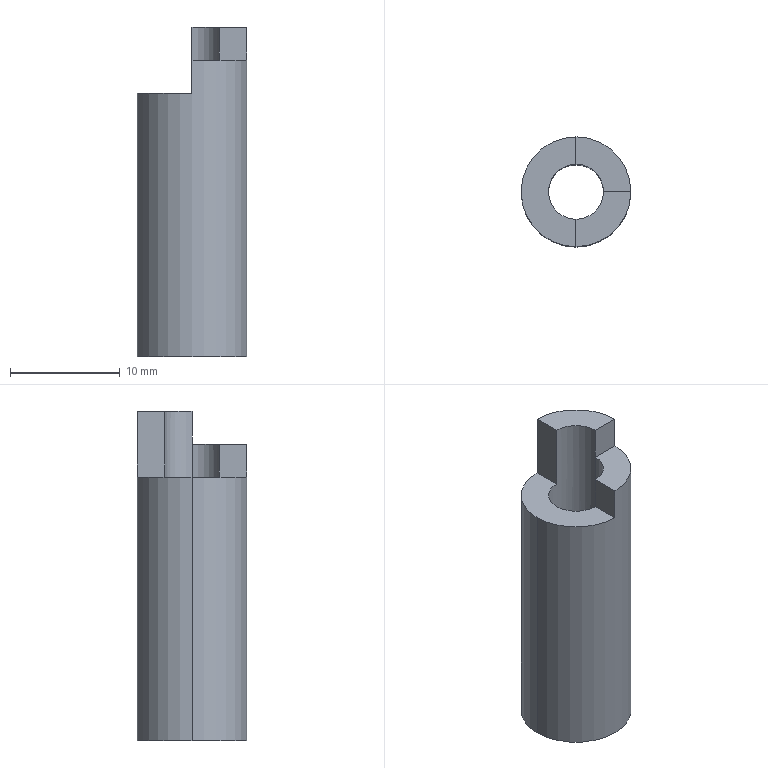Part | SolidWorks | features BaseBody 1 | 1 solid | 11 faces | box 10 x 10 x 30 mm | volume 1546 mm3 | plane 7 | cylinder 4 | commonest cylinder face diameters 5.003 x2 10 x2
STEP:
#1=CARTESIAN_POINT('',(-86.,-22.498,-9.829));
#2=VERTEX_POINT('',#1);
#3=CARTESIAN_POINT('',(-88.501,-25.,-9.829));
#4=VERTEX_POINT('',#3);
#5=CARTESIAN_POINT('',(-86.,-25.,-9.829));
#6=DIRECTION('',(0.,0.,1.));
#7=DIRECTION('',(-1.,0.,0.));
#8=AXIS2_PLACEMENT_3D('',#5,#6,#7);
#9=CIRCLE('',#8,2.502);
#10=EDGE_CURVE('',#2,#4,#9,.T.);
#11=ORIENTED_EDGE('',*,*,#10,.T.);
#12=CARTESIAN_POINT('',(-88.501,-25.,-33.829));
#13=VERTEX_POINT('',#12);
#14=CARTESIAN_POINT('',(-88.501,-25.,-3.829));
#15=DIRECTION('',(0.,0.,-1.));
#16=VECTOR('',#15,1000.);
#17=LINE('',#14,#16);
#18=EDGE_CURVE('',#4,#13,#17,.T.);
#19=ORIENTED_EDGE('',*,*,#18,.T.);
#20=CARTESIAN_POINT('',(-83.498,-25.,-33.829));
#21=VERTEX_POINT('',#20);
#22=CARTESIAN_POINT('',(-86.,-25.,-33.829));
#23=DIRECTION('',(0.,0.,1.));
#24=DIRECTION('',(1.,0.,0.));
#25=AXIS2_PLACEMENT_3D('',#22,#23,#24);
#26=CIRCLE('',#25,2.502);
#27=EDGE_CURVE('',#21,#13,#26,.T.);
#28=ORIENTED_EDGE('',*,*,#27,.F.);
#29=CARTESIAN_POINT('',(-83.499,-25.,-6.829));
#30=VERTEX_POINT('',#29);
#31=CARTESIAN_POINT('',(-83.498,-25.,-3.829));
#32=DIRECTION('',(0.,0.,-1.));
#33=VECTOR('',#32,1000.);
#34=LINE('',#31,#33);
#35=EDGE_CURVE('',#30,#21,#34,.T.);
#36=ORIENTED_EDGE('',*,*,#35,.F.);
#37=CARTESIAN_POINT('',(-83.499,-25.,-3.829));
#38=VERTEX_POINT('',#37);
#39=CARTESIAN_POINT('',(-83.499,-25.,-3.829));
#40=DIRECTION('',(0.,0.,1.));
#41=VECTOR('',#40,1000.);
#42=LINE('',#39,#41);
#43=EDGE_CURVE('',#30,#38,#42,.T.);
#44=ORIENTED_EDGE('',*,*,#43,.T.);
#45=CARTESIAN_POINT('',(-86.,-22.498,-3.829));
#46=VERTEX_POINT('',#45);
#47=CARTESIAN_POINT('',(-86.,-25.,-3.829));
#48=DIRECTION('',(0.,0.,-1.));
#49=DIRECTION('',(1.,0.,0.));
#50=AXIS2_PLACEMENT_3D('',#47,#48,#49);
#51=CIRCLE('',#50,2.502);
#52=EDGE_CURVE('',#46,#38,#51,.T.);
#53=ORIENTED_EDGE('',*,*,#52,.F.);
#54=CARTESIAN_POINT('',(-86.,-22.498,-3.829));
#55=DIRECTION('',(0.,0.,-1.));
#56=VECTOR('',#55,1000.);
#57=LINE('',#54,#56);
#58=EDGE_CURVE('',#46,#2,#57,.T.);
#59=ORIENTED_EDGE('',*,*,#58,.T.);
#60=EDGE_LOOP('',(#11,#19,#28,#36,#44,#53,#59));
#61=FACE_OUTER_BOUND('',#60,.T.);
#62=CARTESIAN_POINT('',(-86.,-25.,-3.829));
#63=DIRECTION('',(0.,0.,-1.));
#64=DIRECTION('',(1.,0.,0.));
#65=AXIS2_PLACEMENT_3D('',#62,#63,#64);
#66=CYLINDRICAL_SURFACE('',#65,2.502);
#67=ADVANCED_FACE('',(#61),#66,.F.);
#68=CARTESIAN_POINT('',(-91.,-25.,-9.829));
#69=VERTEX_POINT('',#68);
#70=CARTESIAN_POINT('',(-86.,-30.,-9.829));
#71=VERTEX_POINT('',#70);
#72=CARTESIAN_POINT('',(-86.,-25.,-9.829));
#73=DIRECTION('',(0.,0.,1.));
#74=DIRECTION('',(-1.,0.,0.));
#75=AXIS2_PLACEMENT_3D('',#72,#73,#74);
#76=CIRCLE('',#75,5.);
#77=EDGE_CURVE('',#69,#71,#76,.T.);
#78=ORIENTED_EDGE('',*,*,#77,.F.);
#79=CARTESIAN_POINT('',(-91.,-25.,-33.829));
#80=VERTEX_POINT('',#79);
#81=CARTESIAN_POINT('',(-91.,-25.,-3.829));
#82=DIRECTION('',(0.,0.,-1.));
#83=VECTOR('',#82,1000.);
#84=LINE('',#81,#83);
#85=EDGE_CURVE('',#69,#80,#84,.T.);
#86=ORIENTED_EDGE('',*,*,#85,.T.);
#87=CARTESIAN_POINT('',(-81.,-25.,-33.829));
#88=VERTEX_POINT('',#87);
#89=CARTESIAN_POINT('',(-86.,-25.,-33.829));
#90=DIRECTION('',(0.,0.,1.));
#91=DIRECTION('',(1.,0.,0.));
#92=AXIS2_PLACEMENT_3D('',#89,#90,#91);
#93=CIRCLE('',#92,5.);
#94=EDGE_CURVE('',#80,#88,#93,.T.);
#95=ORIENTED_EDGE('',*,*,#94,.T.);
#96=CARTESIAN_POINT('',(-81.,-25.,-6.829));
#97=VERTEX_POINT('',#96);
#98=CARTESIAN_POINT('',(-81.,-25.,-3.829));
#99=DIRECTION('',(0.,0.,-1.));
#100=VECTOR('',#99,1000.);
#101=LINE('',#98,#100);
#102=EDGE_CURVE('',#97,#88,#101,.T.);
#103=ORIENTED_EDGE('',*,*,#102,.F.);
#104=CARTESIAN_POINT('',(-86.,-30.,-6.829));
#105=VERTEX_POINT('',#104);
#106=CARTESIAN_POINT('',(-86.,-25.,-6.829));
#107=DIRECTION('',(0.,0.,1.));
#108=DIRECTION('',(-1.,0.,0.));
#109=AXIS2_PLACEMENT_3D('',#106,#107,#108);
#110=CIRCLE('',#109,5.);
#111=EDGE_CURVE('',#105,#97,#110,.T.);
#112=ORIENTED_EDGE('',*,*,#111,.F.);
#113=CARTESIAN_POINT('',(-86.,-30.,-3.829));
#114=DIRECTION('',(0.,0.,1.));
#115=VECTOR('',#114,1000.);
#116=LINE('',#113,#115);
#117=EDGE_CURVE('',#71,#105,#116,.T.);
#118=ORIENTED_EDGE('',*,*,#117,.F.);
#119=EDGE_LOOP('',(#78,#86,#95,#103,#112,#118));
#120=FACE_OUTER_BOUND('',#119,.T.);
#121=CARTESIAN_POINT('',(-86.,-25.,-3.829));
#122=DIRECTION('',(0.,0.,-1.));
#123=DIRECTION('',(1.,0.,0.));
#124=AXIS2_PLACEMENT_3D('',#121,#122,#123);
#125=CYLINDRICAL_SURFACE('',#124,5.);
#126=ADVANCED_FACE('',(#120),#125,.T.);
#127=ORIENTED_EDGE('',*,*,#27,.T.);
#128=CARTESIAN_POINT('',(-86.,-25.,-33.829));
#129=DIRECTION('',(0.,0.,1.));
#130=DIRECTION('',(1.,0.,0.));
#131=AXIS2_PLACEMENT_3D('',#128,#129,#130);
#132=CIRCLE('',#131,2.502);
#133=EDGE_CURVE('',#13,#21,#132,.T.);
#134=ORIENTED_EDGE('',*,*,#133,.T.);
#135=EDGE_LOOP('',(#127,#134));
#136=FACE_BOUND('',#135,.T.);
#137=CARTESIAN_POINT('',(-86.,-25.,-33.829));
#138=DIRECTION('',(0.,0.,1.));
#139=DIRECTION('',(1.,0.,0.));
#140=AXIS2_PLACEMENT_3D('',#137,#138,#139);
#141=CIRCLE('',#140,5.);
#142=EDGE_CURVE('',#88,#80,#141,.T.);
#143=ORIENTED_EDGE('',*,*,#142,.F.);
#144=ORIENTED_EDGE('',*,*,#94,.F.);
#145=EDGE_LOOP('',(#143,#144));
#146=FACE_OUTER_BOUND('',#145,.T.);
#147=CARTESIAN_POINT('',(-86.,-25.,-33.829));
#148=DIRECTION('',(0.,0.,-1.));
#149=DIRECTION('',(-1.,0.,0.));
#150=AXIS2_PLACEMENT_3D('',#147,#148,#149);
#151=PLANE('',#150);
#152=ADVANCED_FACE('',(#136,#146),#151,.T.);
#153=CARTESIAN_POINT('',(-81.,-25.,-3.829));
#154=VERTEX_POINT('',#153);
#155=CARTESIAN_POINT('',(-86.,-25.,-3.829));
#156=DIRECTION('',(1.,0.,0.));
#157=VECTOR('',#156,1000.);
#158=LINE('',#155,#157);
#159=EDGE_CURVE('',#38,#154,#158,.T.);
#160=ORIENTED_EDGE('',*,*,#159,.T.);
#161=CARTESIAN_POINT('',(-86.,-20.,-3.829));
#162=VERTEX_POINT('',#161);
#163=CARTESIAN_POINT('',(-86.,-25.,-3.829));
#164=DIRECTION('',(0.,0.,-1.));
#165=DIRECTION('',(1.,0.,0.));
#166=AXIS2_PLACEMENT_3D('',#163,#164,#165);
#167=CIRCLE('',#166,5.);
#168=EDGE_CURVE('',#162,#154,#167,.T.);
#169=ORIENTED_EDGE('',*,*,#168,.F.);
#170=CARTESIAN_POINT('',(-86.,-25.,-3.829));
#171=DIRECTION('',(0.,-1.,0.));
#172=VECTOR('',#171,1000.);
#173=LINE('',#170,#172);
#174=EDGE_CURVE('',#162,#46,#173,.T.);
#175=ORIENTED_EDGE('',*,*,#174,.T.);
#176=ORIENTED_EDGE('',*,*,#52,.T.);
#177=EDGE_LOOP('',(#160,#169,#175,#176));
#178=FACE_OUTER_BOUND('',#177,.T.);
#179=CARTESIAN_POINT('',(-86.,-25.,-3.829));
#180=DIRECTION('',(0.,0.,1.));
#181=DIRECTION('',(1.,0.,0.));
#182=AXIS2_PLACEMENT_3D('',#179,#180,#181);
#183=PLANE('',#182);
#184=ADVANCED_FACE('',(#178),#183,.T.);
#185=ORIENTED_EDGE('',*,*,#85,.F.);
#186=CARTESIAN_POINT('',(-86.,-20.,-9.829));
#187=VERTEX_POINT('',#186);
#188=CARTESIAN_POINT('',(-86.,-25.,-9.829));
#189=DIRECTION('',(0.,0.,1.));
#190=DIRECTION('',(-1.,0.,0.));
#191=AXIS2_PLACEMENT_3D('',#188,#189,#190);
#192=CIRCLE('',#191,5.);
#193=EDGE_CURVE('',#187,#69,#192,.T.);
#194=ORIENTED_EDGE('',*,*,#193,.F.);
#195=CARTESIAN_POINT('',(-86.,-20.,-3.829));
#196=DIRECTION('',(0.,0.,-1.));
#197=VECTOR('',#196,1000.);
#198=LINE('',#195,#197);
#199=EDGE_CURVE('',#162,#187,#198,.T.);
#200=ORIENTED_EDGE('',*,*,#199,.F.);
#201=ORIENTED_EDGE('',*,*,#168,.T.);
#202=CARTESIAN_POINT('',(-81.,-25.,-3.829));
#203=DIRECTION('',(0.,0.,1.));
#204=VECTOR('',#203,1000.);
#205=LINE('',#202,#204);
#206=EDGE_CURVE('',#97,#154,#205,.T.);
#207=ORIENTED_EDGE('',*,*,#206,.F.);
#208=ORIENTED_EDGE('',*,*,#102,.T.);
#209=ORIENTED_EDGE('',*,*,#142,.T.);
#210=EDGE_LOOP('',(#185,#194,#200,#201,#207,#208,#209));
#211=FACE_OUTER_BOUND('',#210,.T.);
#212=CARTESIAN_POINT('',(-86.,-25.,-3.829));
#213=DIRECTION('',(0.,0.,-1.));
#214=DIRECTION('',(1.,0.,0.));
#215=AXIS2_PLACEMENT_3D('',#212,#213,#214);
#216=CYLINDRICAL_SURFACE('',#215,5.);
#217=ADVANCED_FACE('',(#211),#216,.T.);
#218=ORIENTED_EDGE('',*,*,#18,.F.);
#219=CARTESIAN_POINT('',(-86.,-27.502,-9.829));
#220=VERTEX_POINT('',#219);
#221=CARTESIAN_POINT('',(-86.,-25.,-9.829));
#222=DIRECTION('',(0.,0.,1.));
#223=DIRECTION('',(-1.,0.,0.));
#224=AXIS2_PLACEMENT_3D('',#221,#222,#223);
#225=CIRCLE('',#224,2.502);
#226=EDGE_CURVE('',#4,#220,#225,.T.);
#227=ORIENTED_EDGE('',*,*,#226,.T.);
#228=CARTESIAN_POINT('',(-86.,-27.502,-6.829));
#229=VERTEX_POINT('',#228);
#230=CARTESIAN_POINT('',(-86.,-27.502,-3.829));
#231=DIRECTION('',(0.,0.,1.));
#232=VECTOR('',#231,1000.);
#233=LINE('',#230,#232);
#234=EDGE_CURVE('',#220,#229,#233,.T.);
#235=ORIENTED_EDGE('',*,*,#234,.T.);
#236=CARTESIAN_POINT('',(-86.,-25.,-6.829));
#237=DIRECTION('',(0.,0.,1.));
#238=DIRECTION('',(-1.,0.,0.));
#239=AXIS2_PLACEMENT_3D('',#236,#237,#238);
#240=CIRCLE('',#239,2.502);
#241=EDGE_CURVE('',#229,#30,#240,.T.);
#242=ORIENTED_EDGE('',*,*,#241,.T.);
#243=ORIENTED_EDGE('',*,*,#35,.T.);
#244=ORIENTED_EDGE('',*,*,#133,.F.);
#245=EDGE_LOOP('',(#218,#227,#235,#242,#243,#244));
#246=FACE_OUTER_BOUND('',#245,.T.);
#247=CARTESIAN_POINT('',(-86.,-25.,-3.829));
#248=DIRECTION('',(0.,0.,-1.));
#249=DIRECTION('',(1.,0.,0.));
#250=AXIS2_PLACEMENT_3D('',#247,#248,#249);
#251=CYLINDRICAL_SURFACE('',#250,2.502);
#252=ADVANCED_FACE('',(#246),#251,.F.);
#253=ORIENTED_EDGE('',*,*,#193,.T.);
#254=ORIENTED_EDGE('',*,*,#77,.T.);
#255=CARTESIAN_POINT('',(-86.,-25.,-9.829));
#256=DIRECTION('',(0.,-1.,0.));
#257=VECTOR('',#256,1000.);
#258=LINE('',#255,#257);
#259=EDGE_CURVE('',#220,#71,#258,.T.);
#260=ORIENTED_EDGE('',*,*,#259,.F.);
#261=ORIENTED_EDGE('',*,*,#226,.F.);
#262=ORIENTED_EDGE('',*,*,#10,.F.);
#263=CARTESIAN_POINT('',(-86.,-25.,-9.829));
#264=DIRECTION('',(0.,-1.,0.));
#265=VECTOR('',#264,1000.);
#266=LINE('',#263,#265);
#267=EDGE_CURVE('',#187,#2,#266,.T.);
#268=ORIENTED_EDGE('',*,*,#267,.F.);
#269=EDGE_LOOP('',(#253,#254,#260,#261,#262,#268));
#270=FACE_OUTER_BOUND('',#269,.T.);
#271=CARTESIAN_POINT('',(-89.001,-25.,-9.829));
#272=DIRECTION('',(0.,0.,-1.));
#273=DIRECTION('',(-1.,0.,0.));
#274=AXIS2_PLACEMENT_3D('',#271,#272,#273);
#275=PLANE('',#274);
#276=ADVANCED_FACE('',(#270),#275,.F.);
#277=ORIENTED_EDGE('',*,*,#117,.T.);
#278=CARTESIAN_POINT('',(-86.,-25.,-6.829));
#279=DIRECTION('',(0.,1.,0.));
#280=VECTOR('',#279,1000.);
#281=LINE('',#278,#280);
#282=EDGE_CURVE('',#105,#229,#281,.T.);
#283=ORIENTED_EDGE('',*,*,#282,.T.);
#284=ORIENTED_EDGE('',*,*,#234,.F.);
#285=ORIENTED_EDGE('',*,*,#259,.T.);
#286=EDGE_LOOP('',(#277,#283,#284,#285));
#287=FACE_OUTER_BOUND('',#286,.T.);
#288=CARTESIAN_POINT('',(-86.,-25.,-9.829));
#289=DIRECTION('',(1.,0.,0.));
#290=DIRECTION('',(0.,0.,-1.));
#291=AXIS2_PLACEMENT_3D('',#288,#289,#290);
#292=PLANE('',#291);
#293=ADVANCED_FACE('',(#287),#292,.F.);
#294=ORIENTED_EDGE('',*,*,#199,.T.);
#295=ORIENTED_EDGE('',*,*,#267,.T.);
#296=ORIENTED_EDGE('',*,*,#58,.F.);
#297=ORIENTED_EDGE('',*,*,#174,.F.);
#298=EDGE_LOOP('',(#294,#295,#296,#297));
#299=FACE_OUTER_BOUND('',#298,.T.);
#300=CARTESIAN_POINT('',(-86.,-25.,-9.829));
#301=DIRECTION('',(1.,0.,0.));
#302=DIRECTION('',(0.,0.,-1.));
#303=AXIS2_PLACEMENT_3D('',#300,#301,#302);
#304=PLANE('',#303);
#305=ADVANCED_FACE('',(#299),#304,.F.);
#306=ORIENTED_EDGE('',*,*,#206,.T.);
#307=ORIENTED_EDGE('',*,*,#159,.F.);
#308=ORIENTED_EDGE('',*,*,#43,.F.);
#309=CARTESIAN_POINT('',(-86.,-25.,-6.829));
#310=DIRECTION('',(1.,0.,0.));
#311=VECTOR('',#310,1000.);
#312=LINE('',#309,#311);
#313=EDGE_CURVE('',#30,#97,#312,.T.);
#314=ORIENTED_EDGE('',*,*,#313,.T.);
#315=EDGE_LOOP('',(#306,#307,#308,#314));
#316=FACE_OUTER_BOUND('',#315,.T.);
#317=CARTESIAN_POINT('',(-86.,-25.,-6.829));
#318=DIRECTION('',(0.,1.,0.));
#319=DIRECTION('',(0.,0.,1.));
#320=AXIS2_PLACEMENT_3D('',#317,#318,#319);
#321=PLANE('',#320);
#322=ADVANCED_FACE('',(#316),#321,.F.);
#323=ORIENTED_EDGE('',*,*,#111,.T.);
#324=ORIENTED_EDGE('',*,*,#313,.F.);
#325=ORIENTED_EDGE('',*,*,#241,.F.);
#326=ORIENTED_EDGE('',*,*,#282,.F.);
#327=EDGE_LOOP('',(#323,#324,#325,#326));
#328=FACE_OUTER_BOUND('',#327,.T.);
#329=CARTESIAN_POINT('',(-86.,-28.002,-6.829));
#330=DIRECTION('',(0.,0.,-1.));
#331=DIRECTION('',(-1.,0.,0.));
#332=AXIS2_PLACEMENT_3D('',#329,#330,#331);
#333=PLANE('',#332);
#334=ADVANCED_FACE('',(#328),#333,.F.);
#335=CLOSED_SHELL('',(#67,#126,#152,#184,#217,#252,#276,#293,#305,#322,#334));
#336=MANIFOLD_SOLID_BREP('',#335);
#337=CARTESIAN_POINT('',(0.,0.,0.));
#338=DIRECTION('',(0.,0.,1.));
#339=DIRECTION('',(1.,0.,0.));
#340=AXIS2_PLACEMENT_3D('',#337,#338,#339);
#341=(LENGTH_UNIT()NAMED_UNIT(*)SI_UNIT(.MILLI.,.METRE.));
#342=UNCERTAINTY_MEASURE_WITH_UNIT(LENGTH_MEASURE(0.00001),#341,'','');
#343=(NAMED_UNIT(*)PLANE_ANGLE_UNIT()SI_UNIT($,.RADIAN.));
#344=(NAMED_UNIT(*)SI_UNIT($,.STERADIAN.)SOLID_ANGLE_UNIT());
#345=(GEOMETRIC_REPRESENTATION_CONTEXT(3)GLOBAL_UNCERTAINTY_ASSIGNED_CONTEXT((#342))GLOBAL_UNIT_ASSIGNED_CONTEXT((#341,#343,#344))REPRESENTATION_CONTEXT('',''));
#346=ADVANCED_BREP_SHAPE_REPRESENTATION('',(#336,#340),#345);